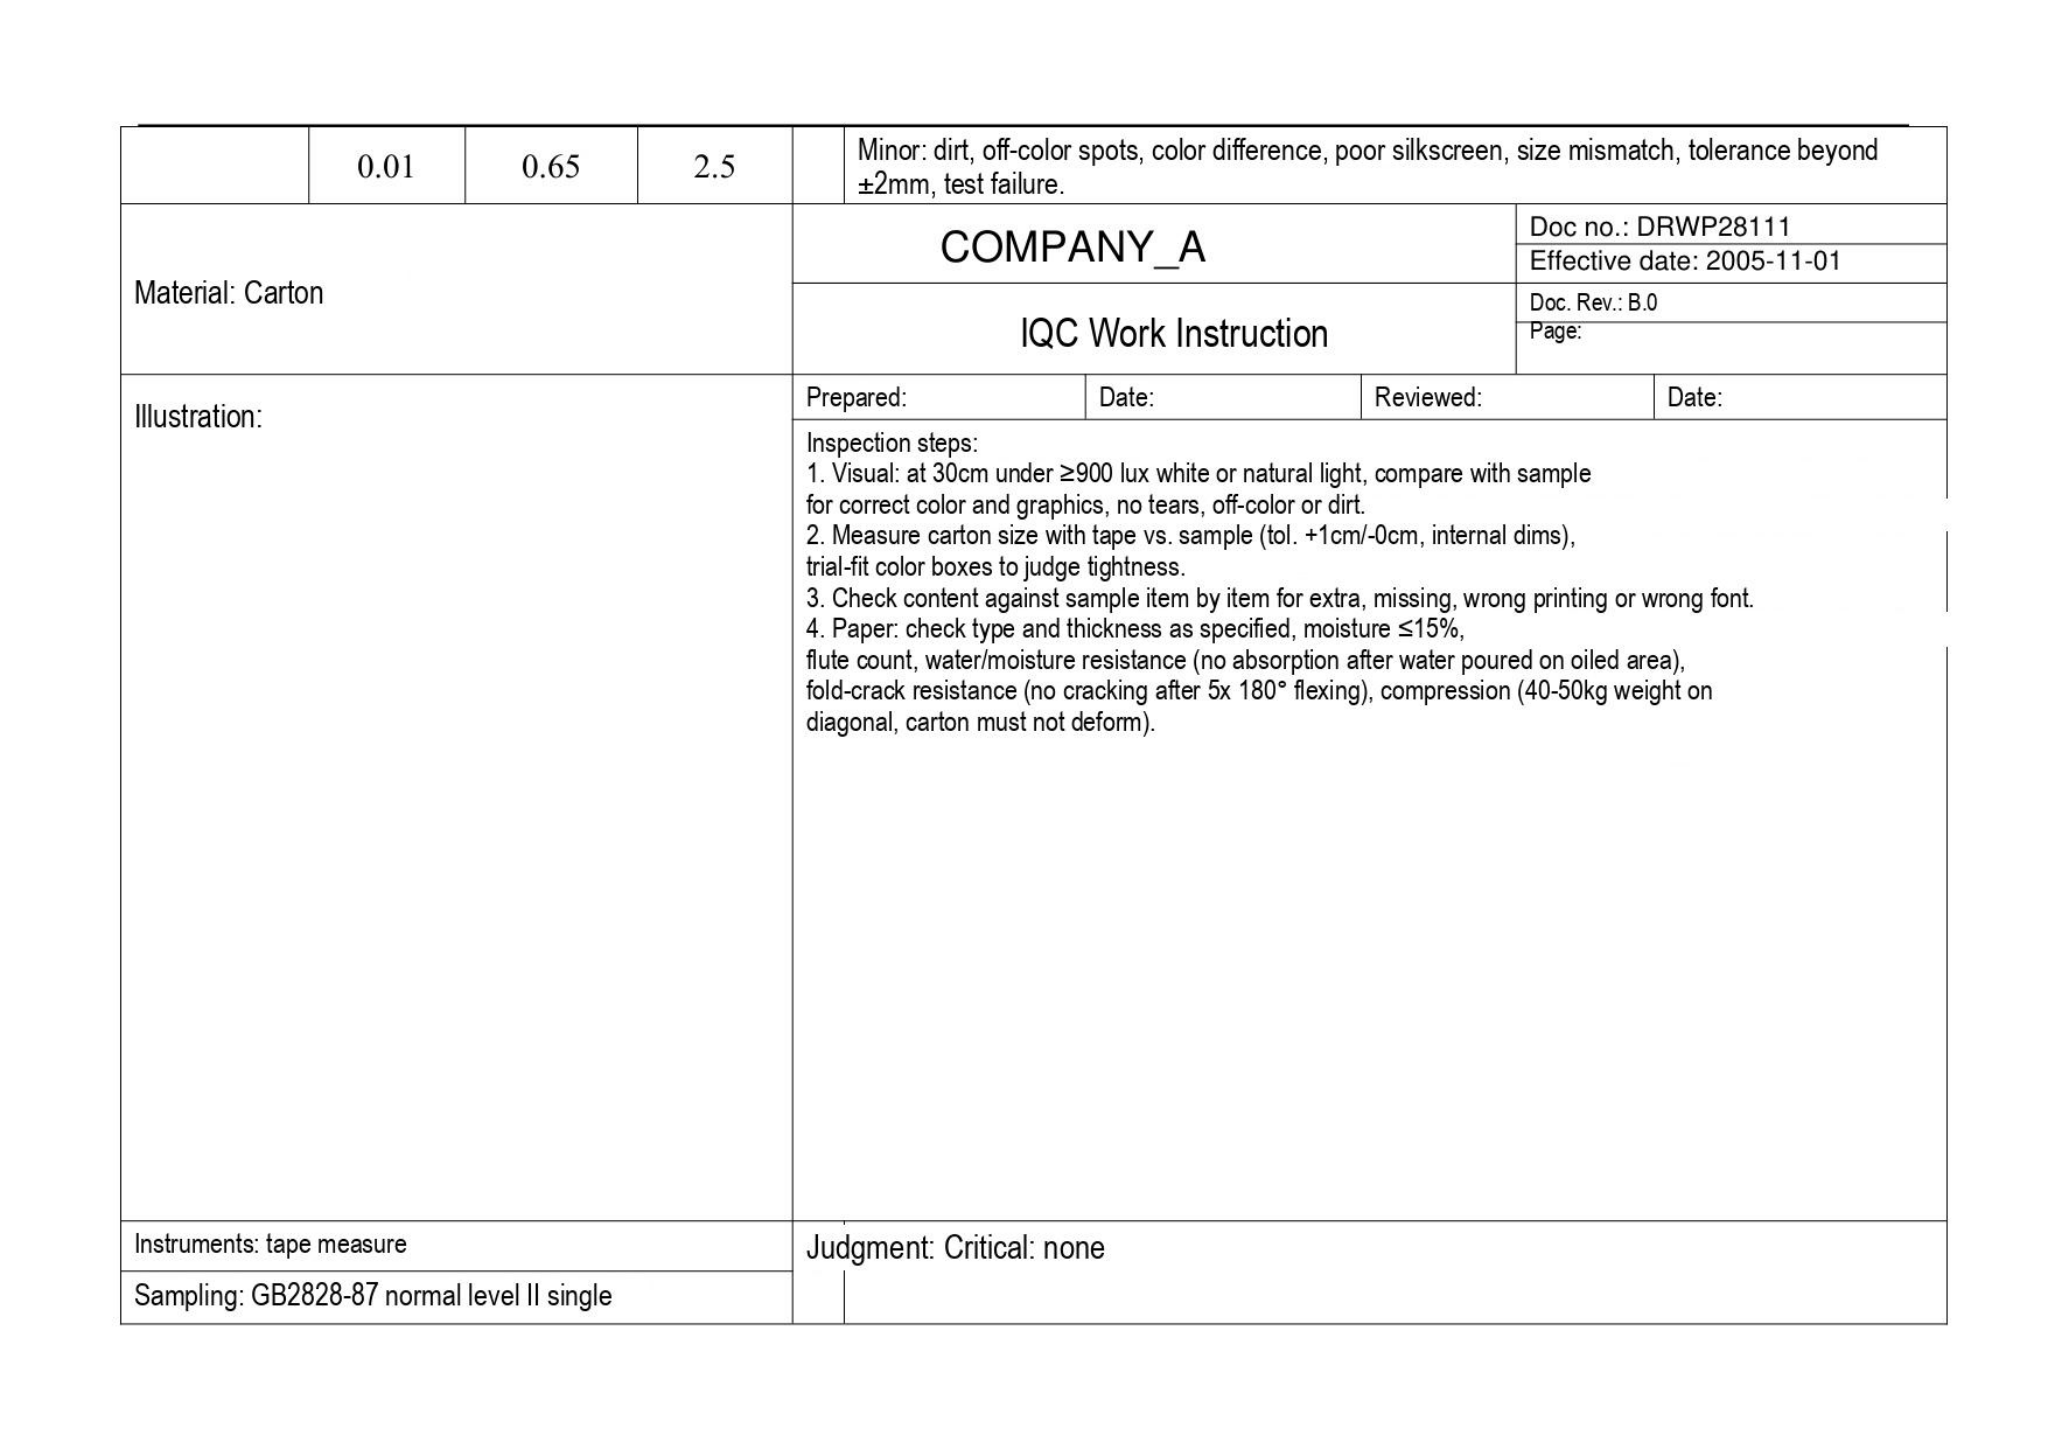| | 0.01 | 0.65 | 2.5 | | Minor: dirt, off-color spots, color difference, poor silkscreen, size mismatch, tolerance beyond ±2mm, test failure. |
|---|---|---|---|---|---|

Material: Carton

COMPANY_A

IQC Work Instruction

Doc no.: DRWP28111
Effective date: 2005-11-01
Doc. Rev.: B.0
Page:

Illustration:

| Prepared: | Date: | Reviewed: | Date: |
|---|---|---|---|

Inspection steps:
1. Visual: at 30cm under ≥900 lux white or natural light, compare with sample for correct color and graphics, no tears, off-color or dirt.
2. Measure carton size with tape vs. sample (tol. +1cm/-0cm, internal dims), trial-fit color boxes to judge tightness.
3. Check content against sample item by item for extra, missing, wrong printing or wrong font.
4. Paper: check type and thickness as specified, moisture ≤15%, flute count, water/moisture resistance (no absorption after water poured on oiled area), fold-crack resistance (no cracking after 5x 180° flexing), compression (40-50kg weight on diagonal, carton must not deform).

Instruments: tape measure

Sampling: GB2828-87 normal level II single

Judgment: Critical: none
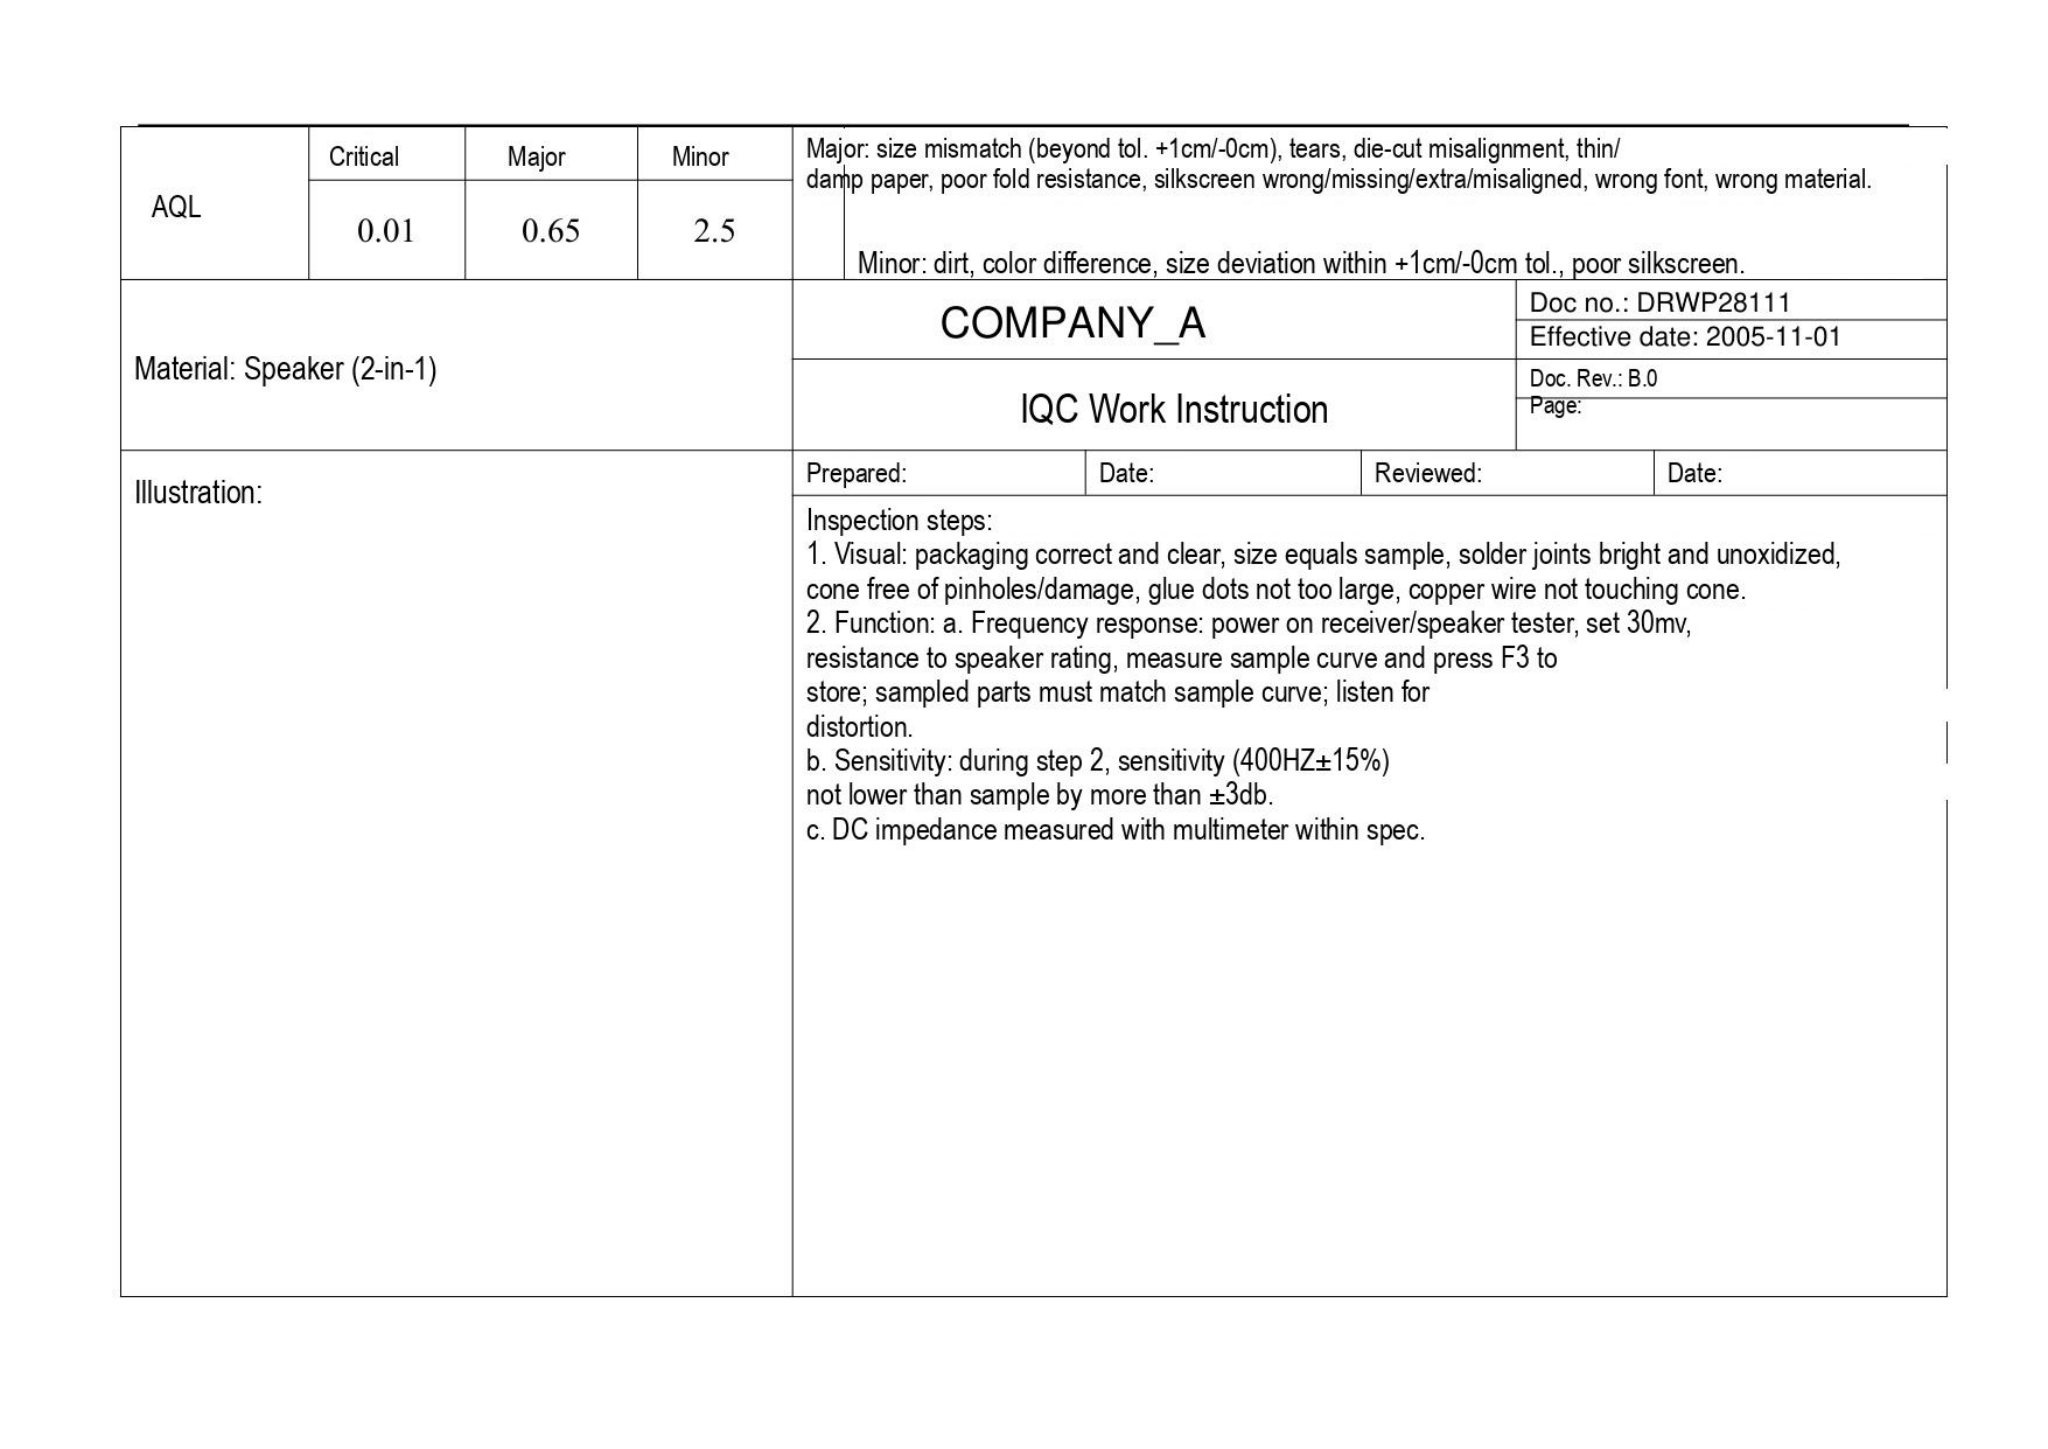| AQL | Critical | Major | Minor |
|---|---|---|---|
| | 0.01 | 0.65 | 2.5 |

Major: size mismatch (beyond tol. +1cm/-0cm), tears, die-cut misalignment, thin/damp paper, poor fold resistance, silkscreen wrong/missing/extra/misaligned, wrong font, wrong material.

Minor: dirt, color difference, size deviation within +1cm/-0cm tol., poor silkscreen.

Material: Speaker (2-in-1)

| COMPANY_A | Doc no.: DRWP28111 |
|---|---|
| | Effective date: 2005-11-01 |
| IQC Work Instruction | Doc. Rev.: B.0 |
| | Page: |

Illustration:

| Prepared: | Date: | Reviewed: | Date: |
|---|---|---|---|

Inspection steps:
1. Visual: packaging correct and clear, size equals sample, solder joints bright and unoxidized, cone free of pinholes/damage, glue dots not too large, copper wire not touching cone.
2. Function: a. Frequency response: power on receiver/speaker tester, set 30mv, resistance to speaker rating, measure sample curve and press F3 to store; sampled parts must match sample curve; listen for distortion.
b. Sensitivity: during step 2, sensitivity (400HZ±15%) not lower than sample by more than ±3db.
c. DC impedance measured with multimeter within spec.
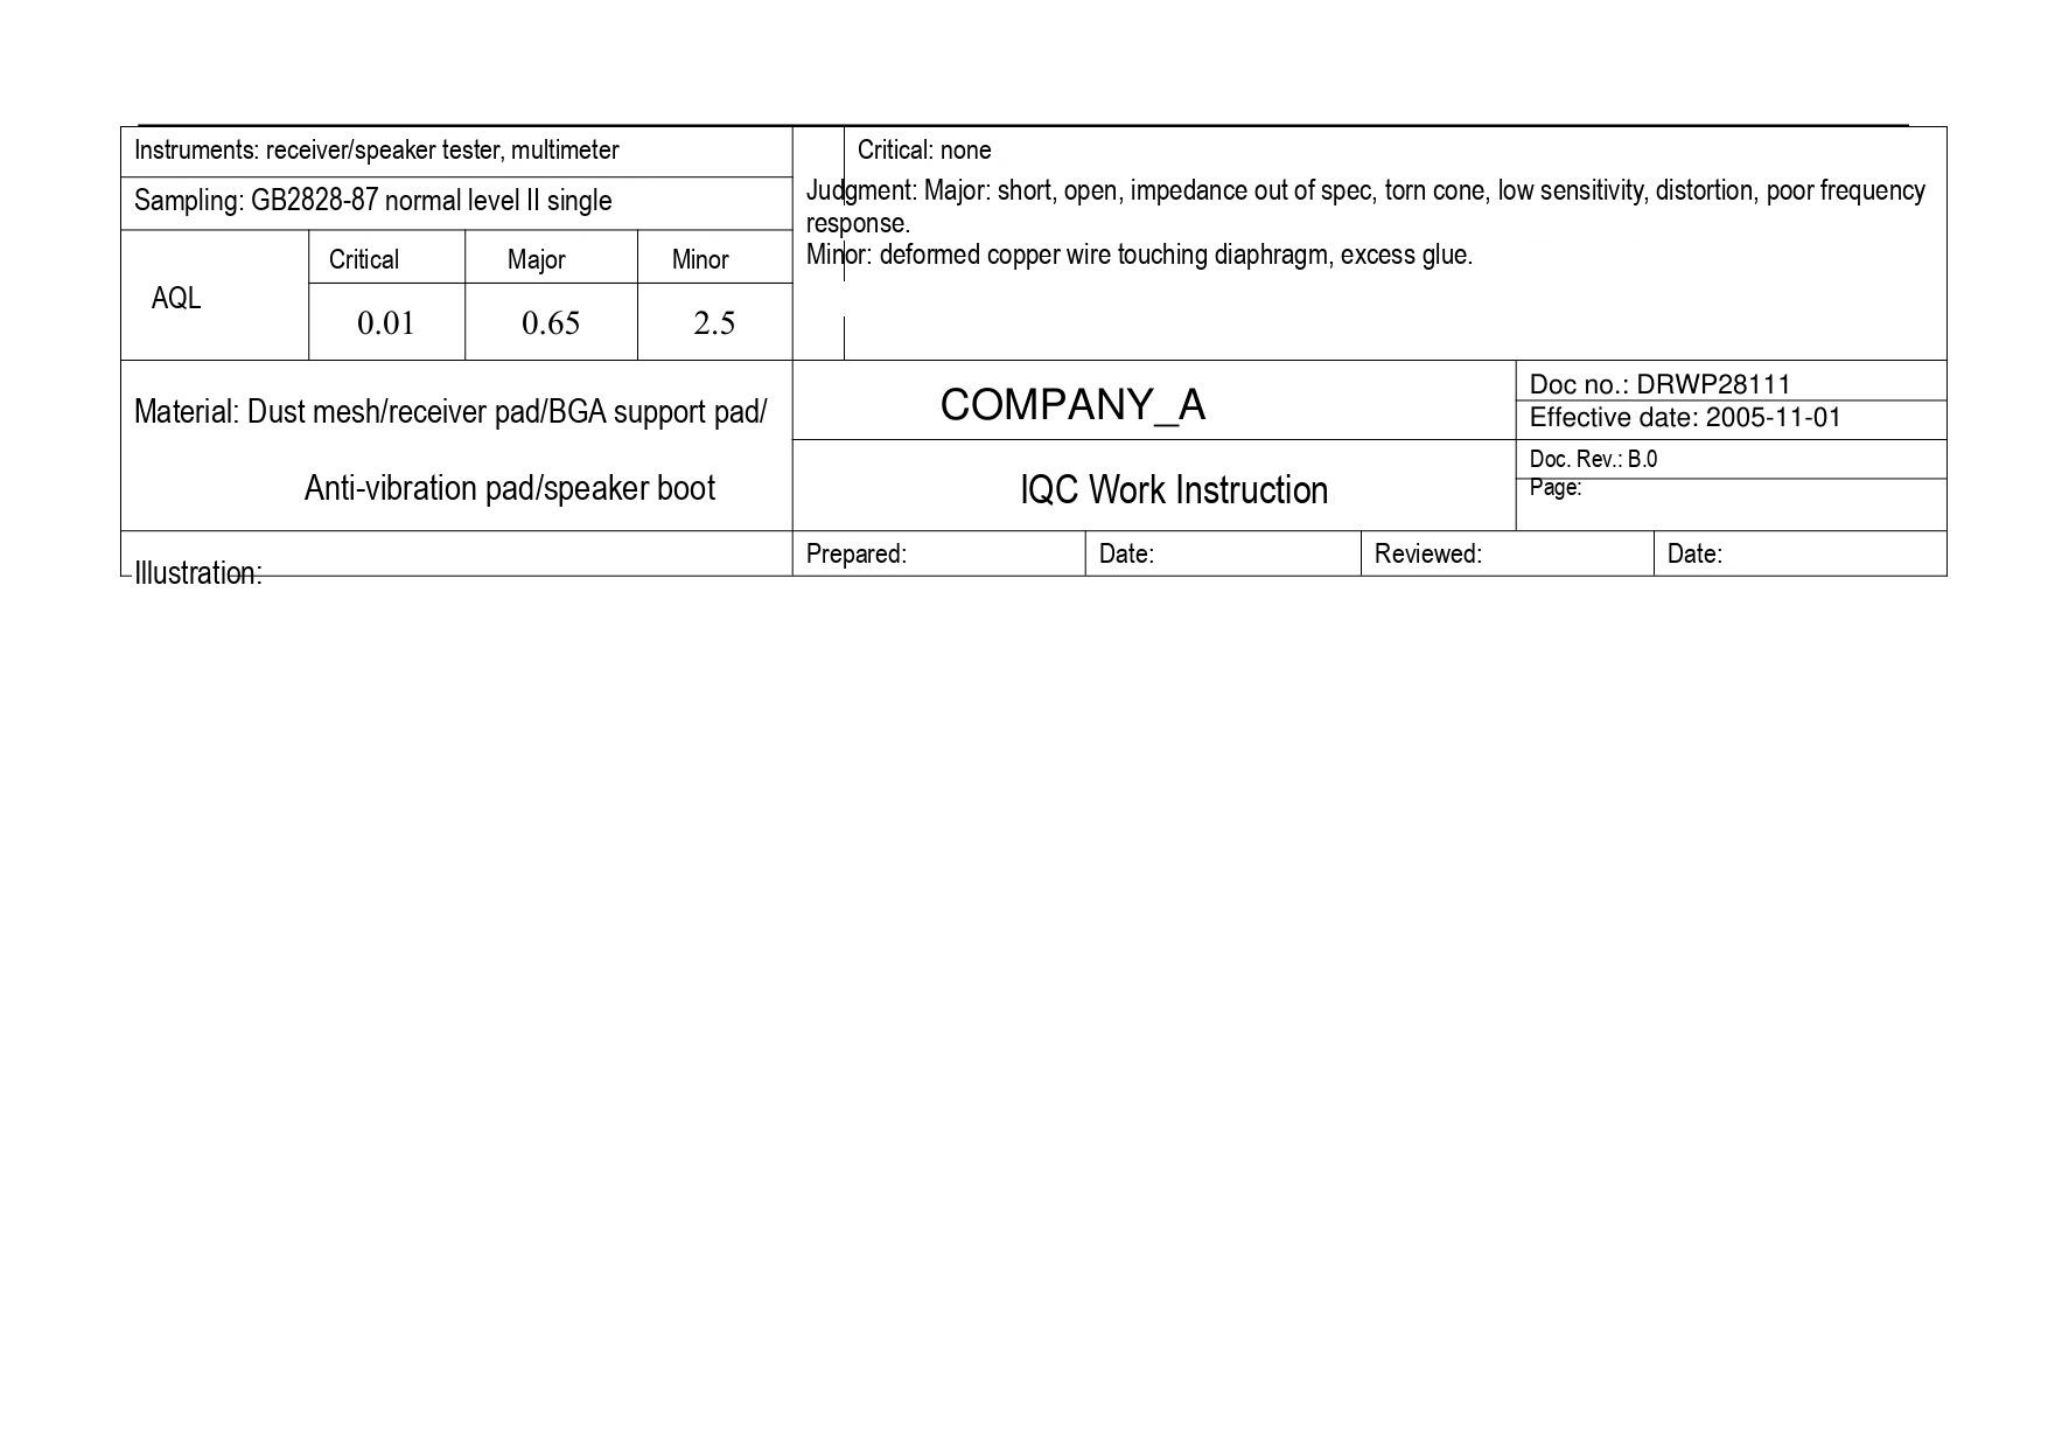Instruments: receiver/speaker tester, multimeter

Sampling: GB2828-87 normal level II single

| AQL | Critical | Major | Minor |
|---|---|---|---|
| | 0.01 | 0.65 | 2.5 |

Critical: none

Judgment: Major: short, open, impedance out of spec, torn cone, low sensitivity, distortion, poor frequency response.
Minor: deformed copper wire touching diaphragm, excess glue.

Material: Dust mesh/receiver pad/BGA support pad/
Anti-vibration pad/speaker boot

COMPANY_A

IQC Work Instruction

Doc no.: DRWP28111
Effective date: 2005-11-01
Doc. Rev.: B.0
Page:

| Prepared: | Date: | Reviewed: | Date: |
|---|---|---|---|

Illustration: Photo-based illustration: receiver/speaker types and their visual standards.
Continued on subsequent page(s).
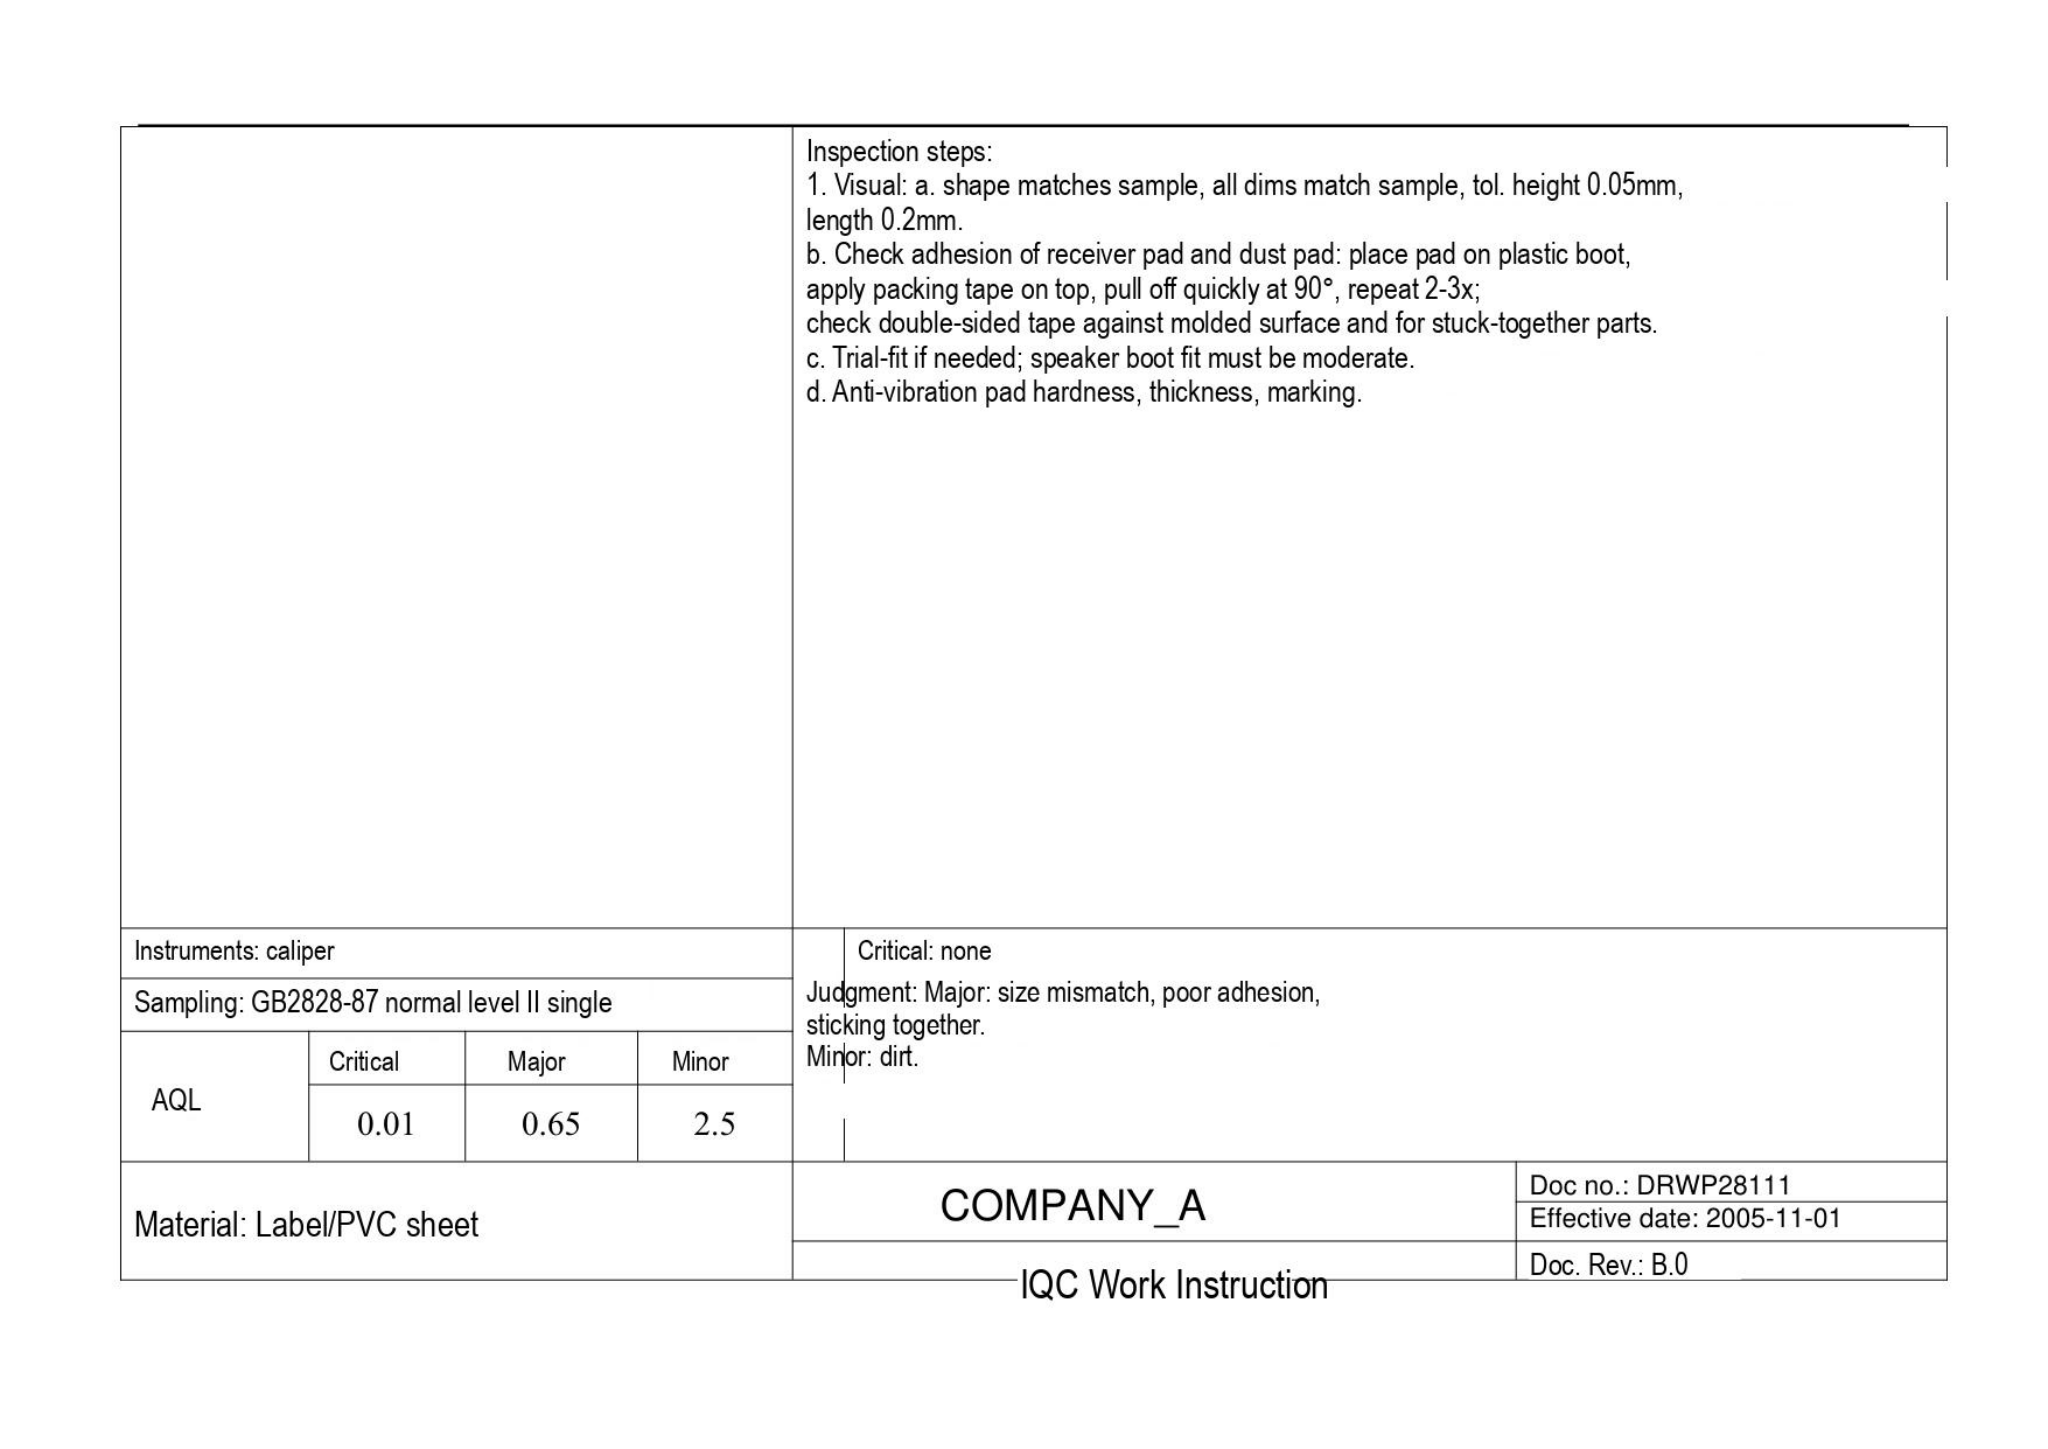Inspection steps:
1. Visual: a. shape matches sample, all dims match sample, tol. height 0.05mm, length 0.2mm.
b. Check adhesion of receiver pad and dust pad: place pad on plastic boot, apply packing tape on top, pull off quickly at 90°, repeat 2-3x;
check double-sided tape against molded surface and for stuck-together parts.
c. Trial-fit if needed; speaker boot fit must be moderate.
d. Anti-vibration pad hardness, thickness, marking.

Instruments: caliper

Sampling: GB2828-87 normal level II single

| AQL | Critical | Major | Minor |
|---|---|---|---|
| | 0.01 | 0.65 | 2.5 |

Critical: none
Judgment: Major: size mismatch, poor adhesion, sticking together.
Minor: dirt.

Material: Label/PVC sheet

COMPANY_A

IQC Work Instruction

Doc no.: DRWP28111
Effective date: 2005-11-01
Doc. Rev.: B.0
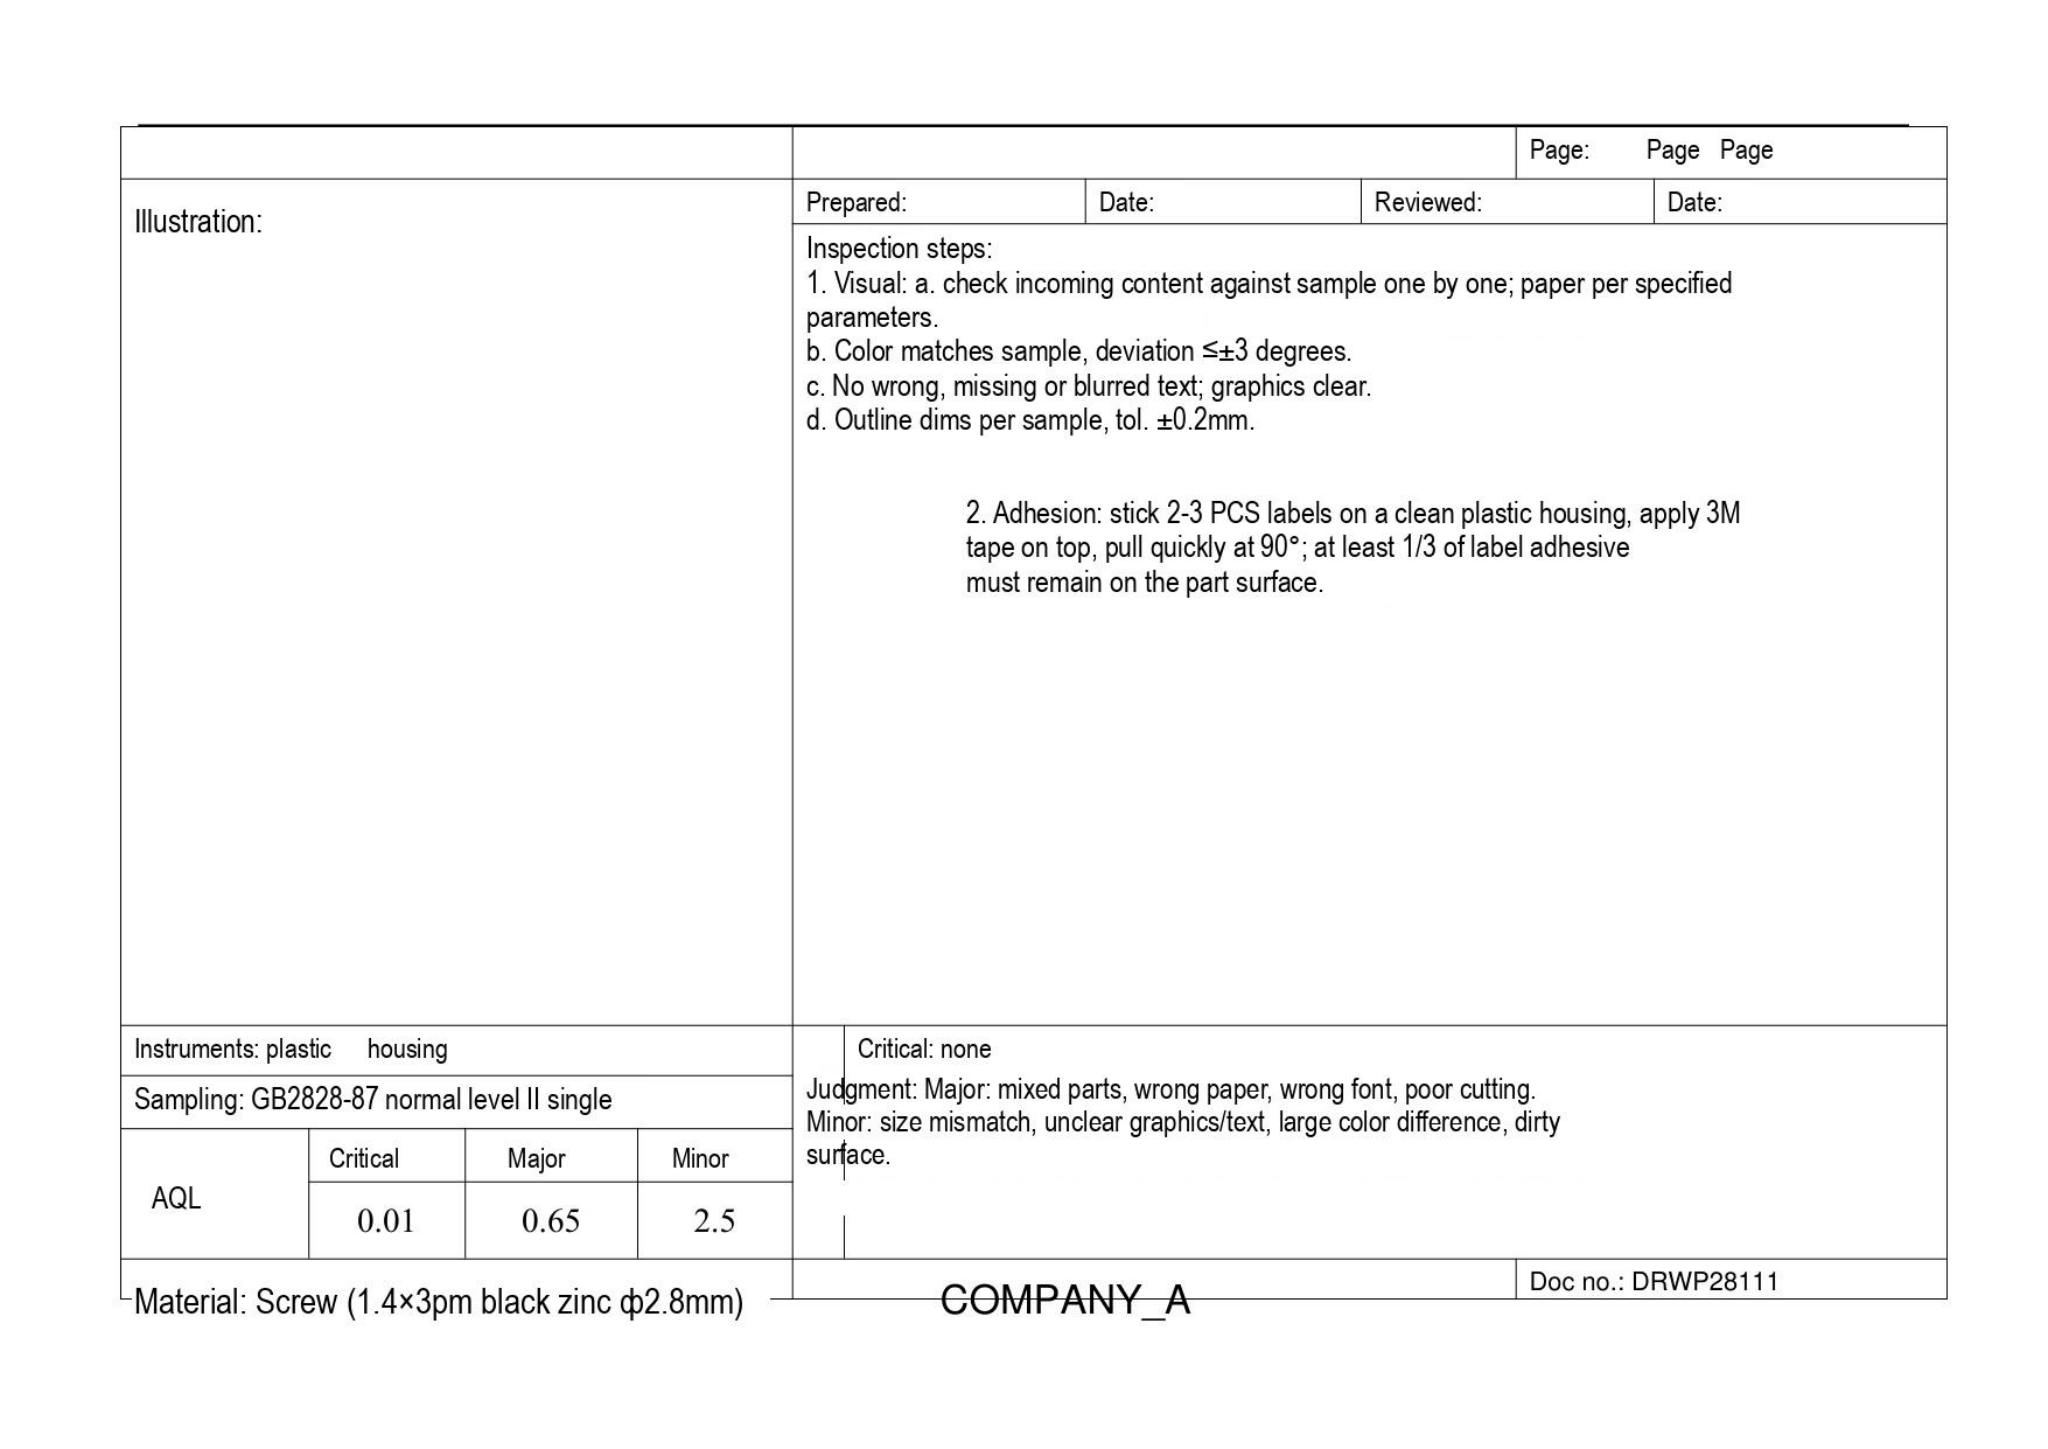Page: Page Page

| Prepared: | Date: | Reviewed: | Date: |
|---|---|---|---|

Illustration:

Inspection steps:
1. Visual: a. check incoming content against sample one by one; paper per specified parameters.
b. Color matches sample, deviation ≤±3 degrees.
c. No wrong, missing or blurred text; graphics clear.
d. Outline dims per sample, tol. ±0.2mm.

2. Adhesion: stick 2-3 PCS labels on a clean plastic housing, apply 3M tape on top, pull quickly at 90°; at least 1/3 of label adhesive must remain on the part surface.

Instruments: plastic housing

Sampling: GB2828-87 normal level II single

| AQL | Critical | Major | Minor |
|---|---|---|---|
| | 0.01 | 0.65 | 2.5 |

Critical: none
Judgment: Major: mixed parts, wrong paper, wrong font, poor cutting.
Minor: size mismatch, unclear graphics/text, large color difference, dirty surface.

Material: Screw (1.4×3pm black zinc ф2.8mm)

COMPANY_A

Doc no.: DRWP28111
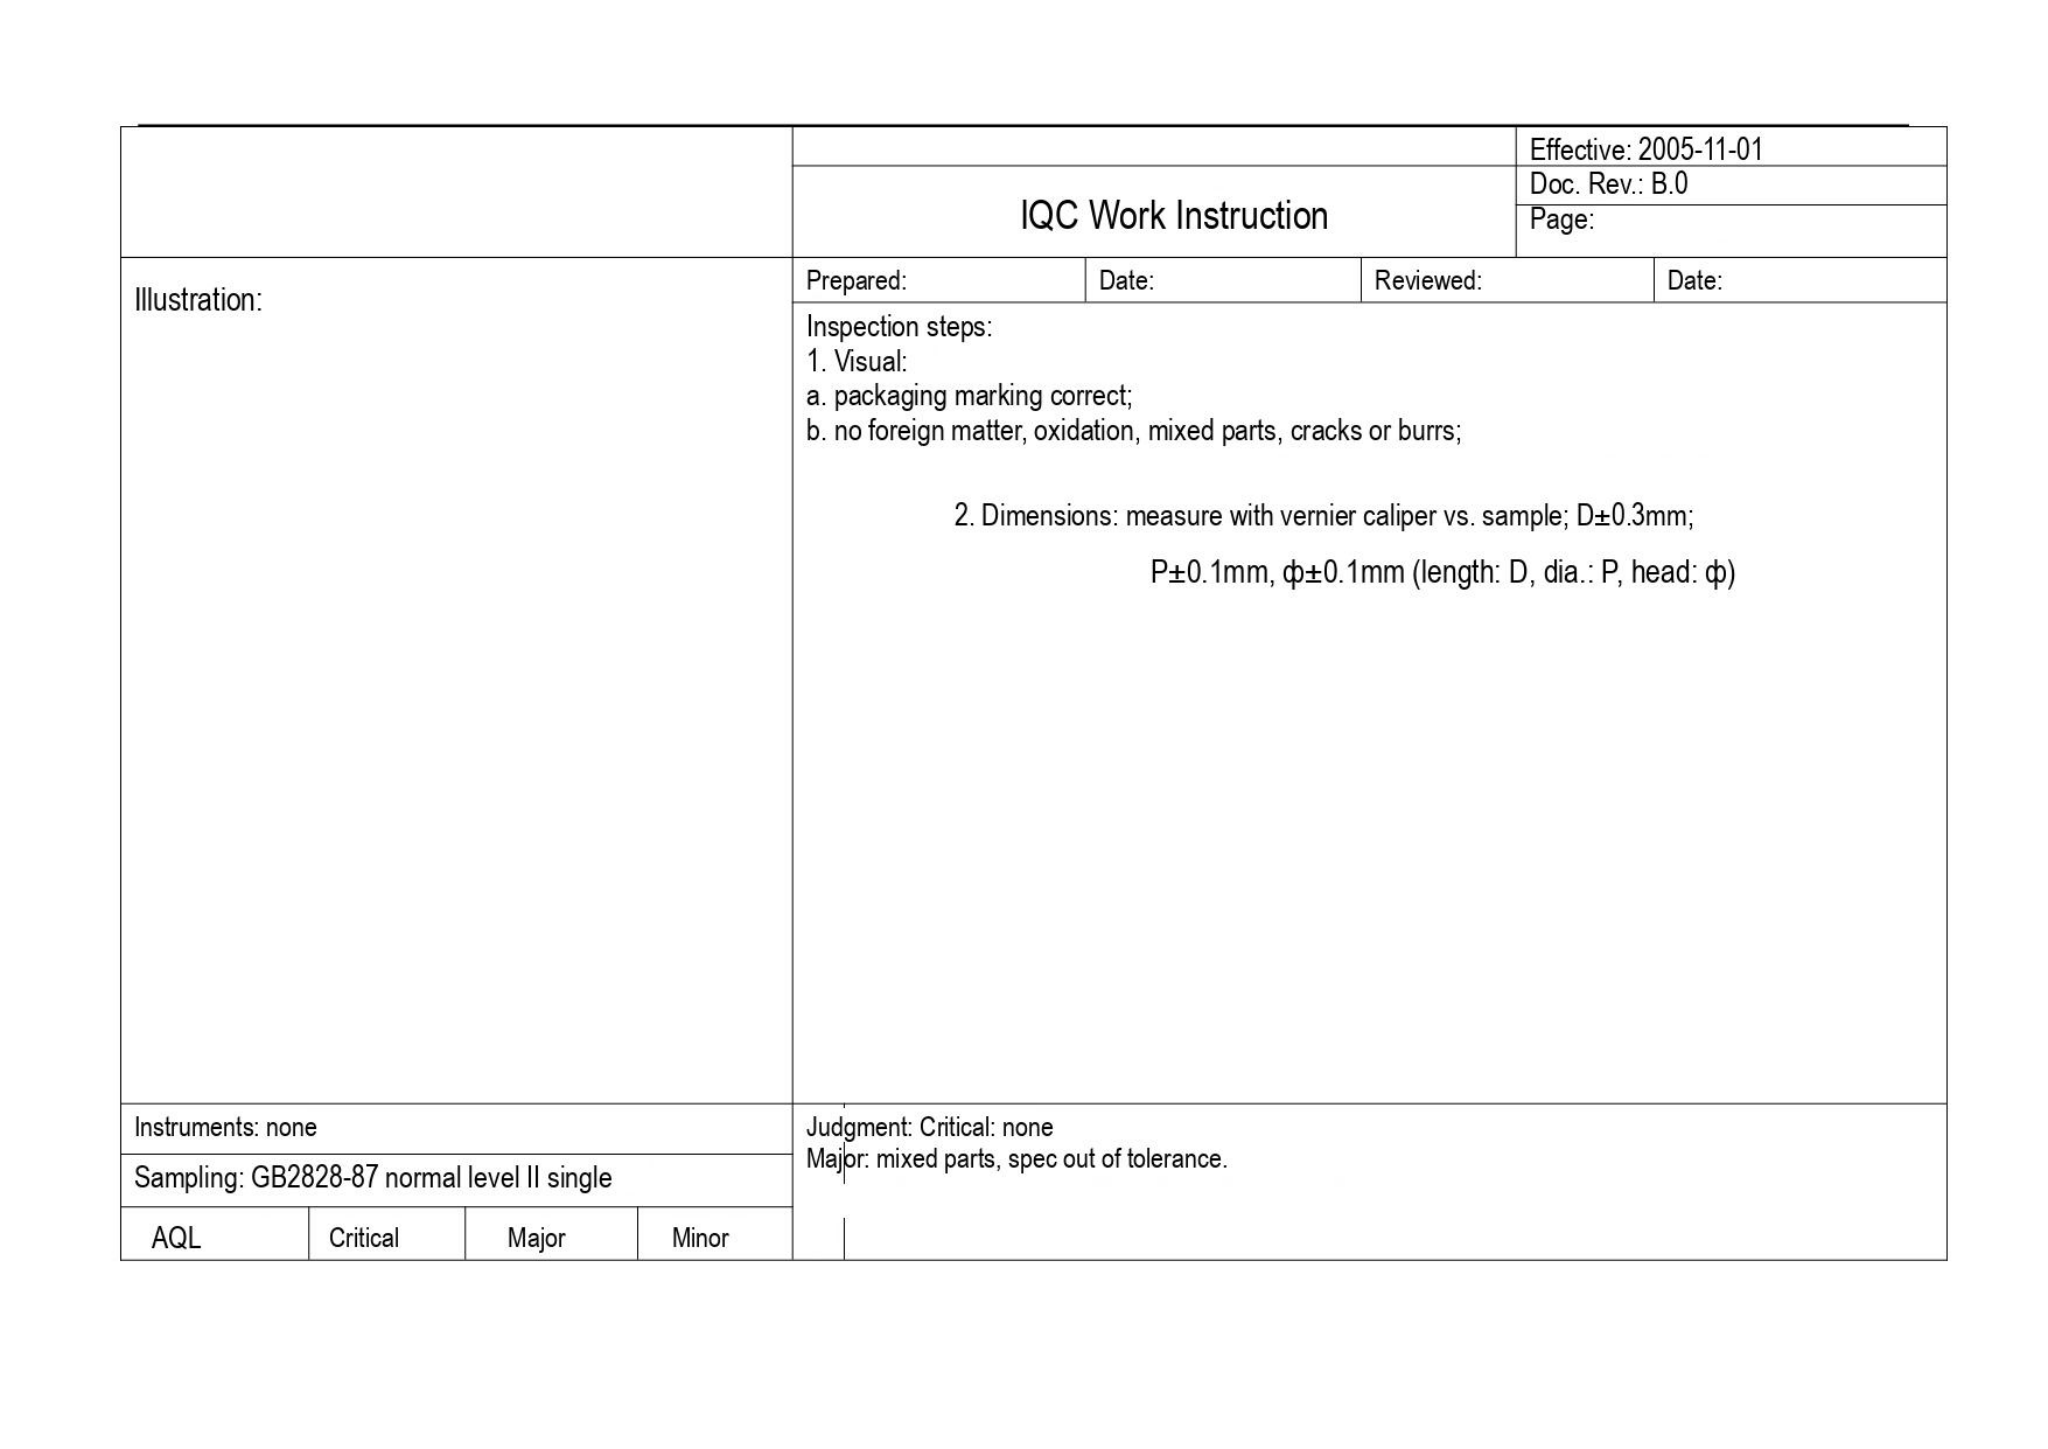IQC Work Instruction

Effective: 2005-11-01
Doc. Rev.: B.0
Page:

| Prepared: | Date: | Reviewed: | Date: |
|---|---|---|---|

Illustration:

Inspection steps:
1. Visual:
a. packaging marking correct;
b. no foreign matter, oxidation, mixed parts, cracks or burrs;

2. Dimensions: measure with vernier caliper vs. sample; D±0.3mm;
P±0.1mm, ф±0.1mm (length: D, dia.: P, head: ф)

Instruments: none

Sampling: GB2828-87 normal level II single

| AQL | Critical | Major | Minor |
|---|---|---|---|

Judgment: Critical: none
Major: mixed parts, spec out of tolerance.
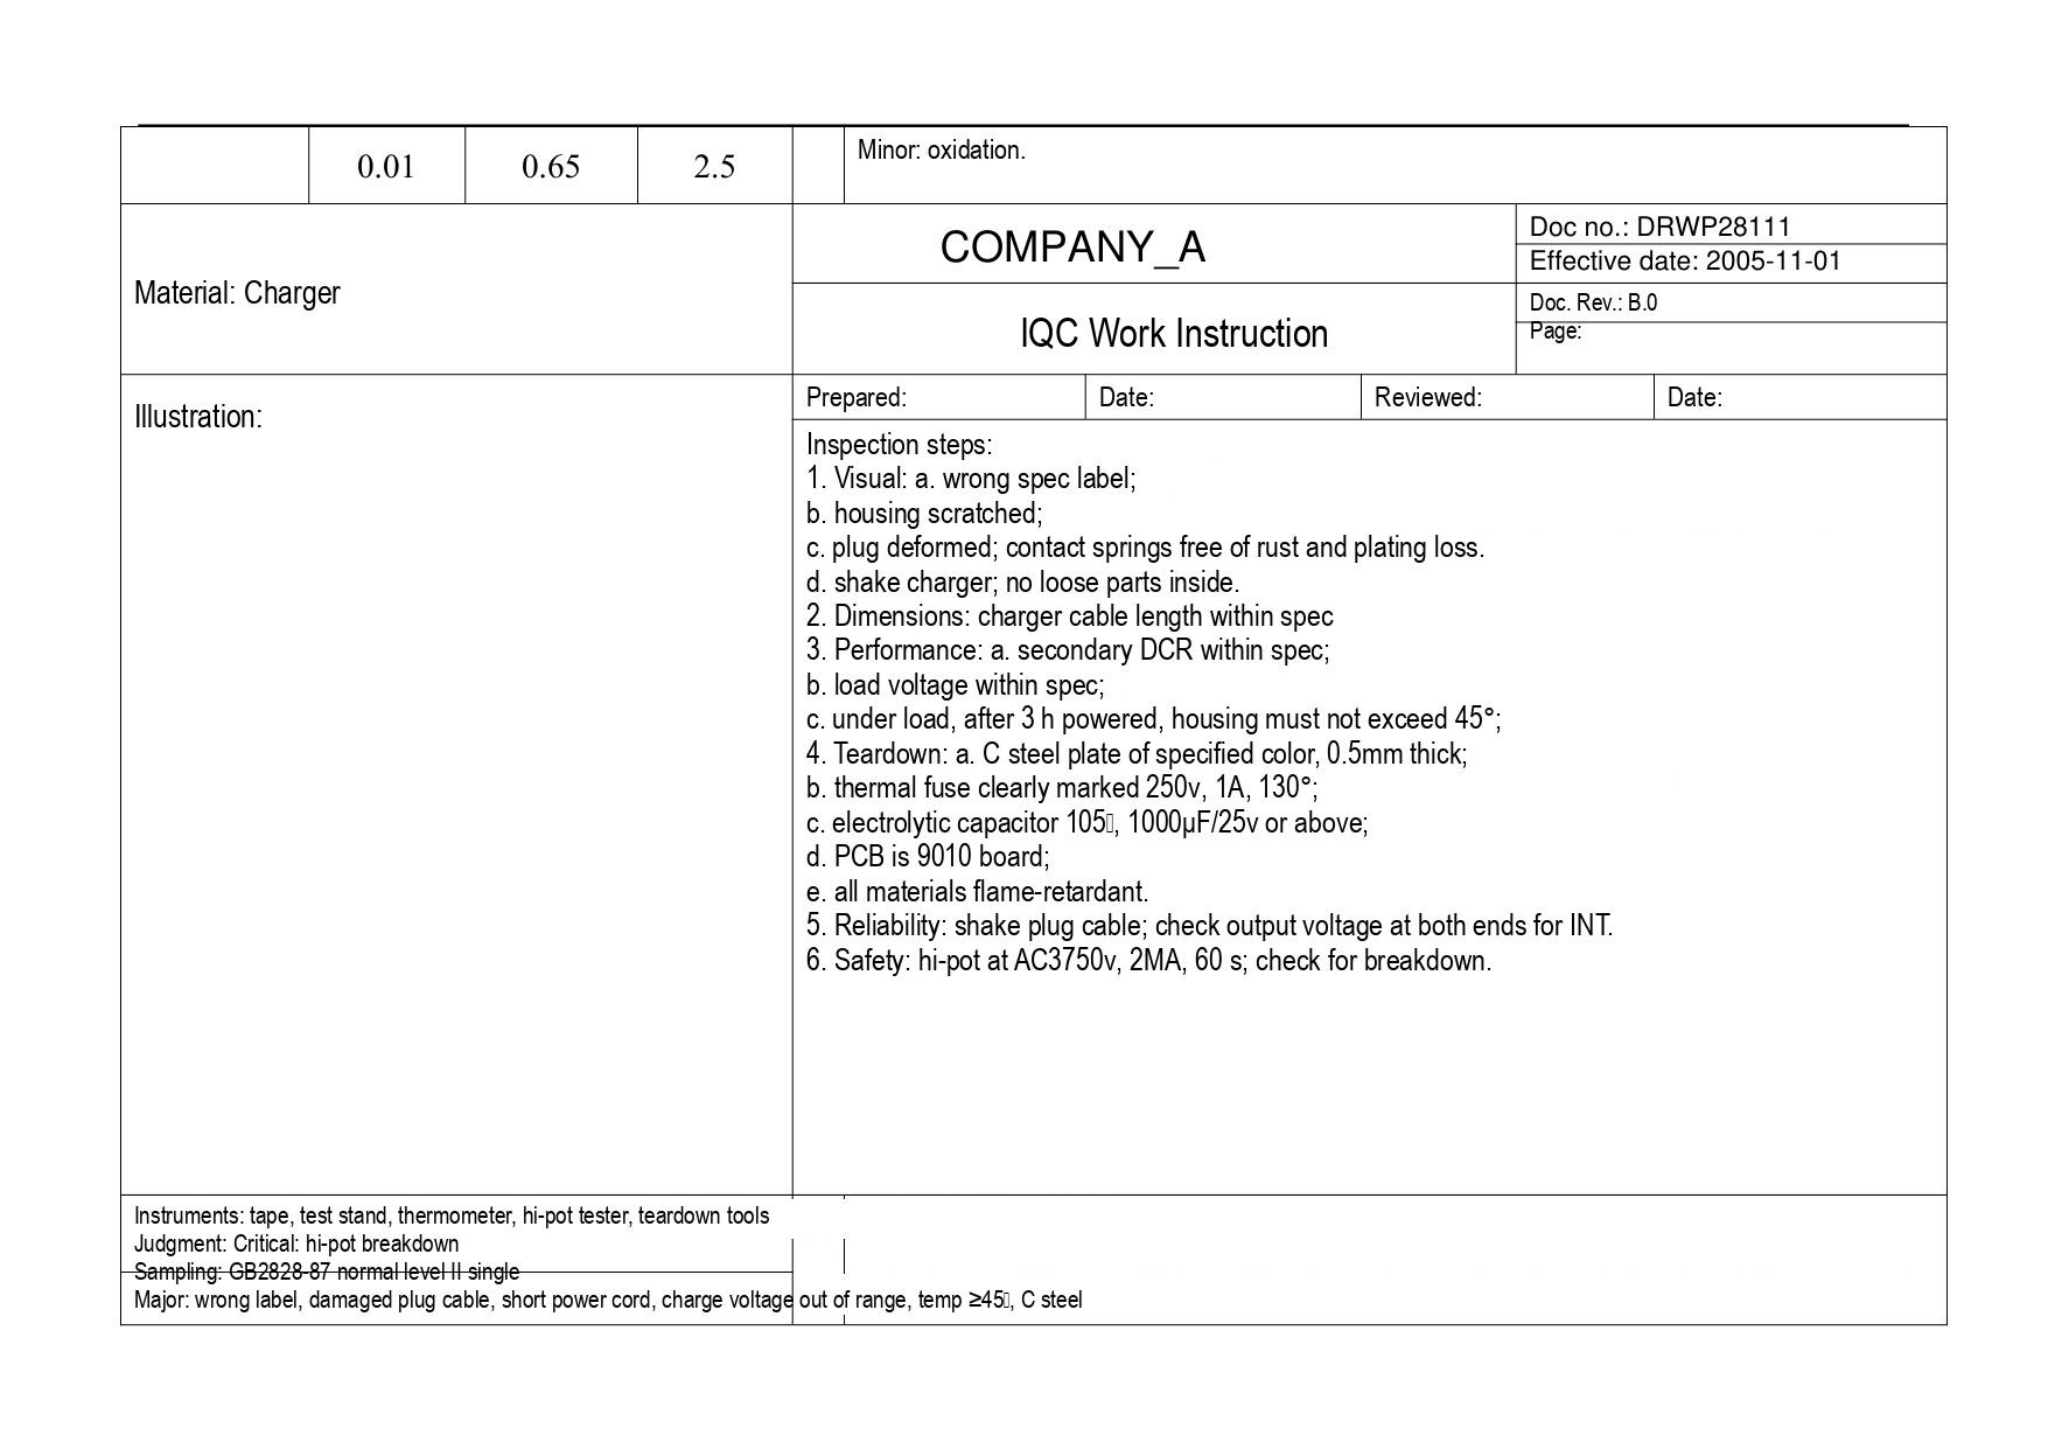| | 0.01 | 0.65 | 2.5 | | Minor: oxidation. |
|---|---|---|---|---|---|

| Material: Charger | COMPANY_A | Doc no.: DRWP28111 |
|---|---|---|
| | | Effective date: 2005-11-01 |
| | IQC Work Instruction | Doc. Rev.: B.0 |
| | | Page: |

Illustration:

| Prepared: | Date: | Reviewed: | Date: |
|---|---|---|---|

Inspection steps:
1. Visual: a. wrong spec label;
b. housing scratched;
c. plug deformed; contact springs free of rust and plating loss.
d. shake charger; no loose parts inside.
2. Dimensions: charger cable length within spec
3. Performance: a. secondary DCR within spec;
b. load voltage within spec;
c. under load, after 3 h powered, housing must not exceed 45°;
4. Teardown: a. C steel plate of specified color, 0.5mm thick;
b. thermal fuse clearly marked 250v, 1A, 130°;
c. electrolytic capacitor 105, 1000μF/25v or above;
d. PCB is 9010 board;
e. all materials flame-retardant.
5. Reliability: shake plug cable; check output voltage at both ends for INT.
6. Safety: hi-pot at AC3750v, 2MA, 60 s; check for breakdown.

Instruments: tape, test stand, thermometer, hi-pot tester, teardown tools
Judgment: Critical: hi-pot breakdown
Sampling: GB2828-87 normal level II single
Major: wrong label, damaged plug cable, short power cord, charge voltage out of range, temp ≥45, C steel